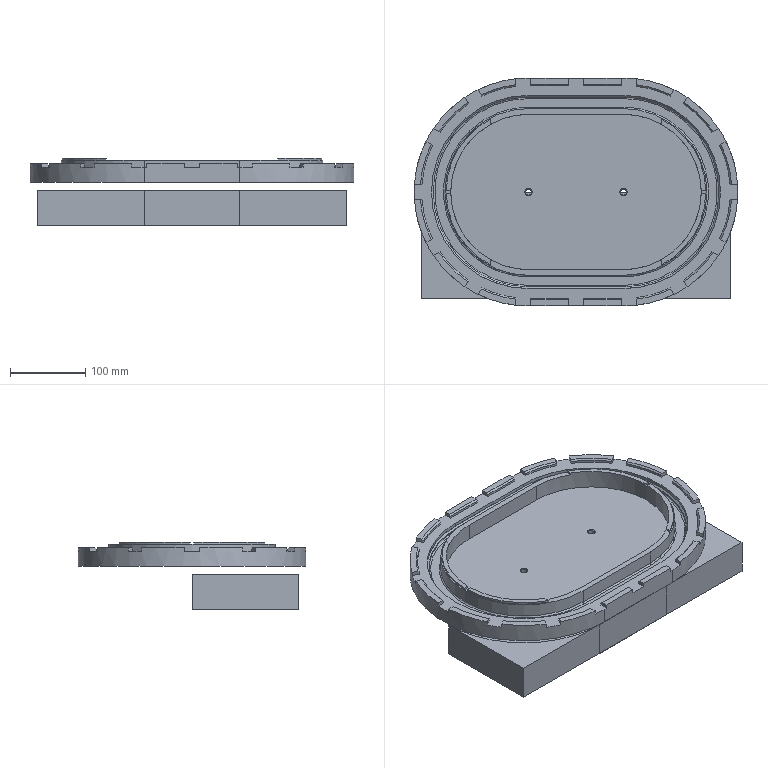NC program | NX | posted with a generic post | part box 429 x 302 x 89.371 mm
Lines 33357 to 34094 of 53366:
(ADAPTIVE_MILLING_COPY , TOOL : D8平刀)
N66710 M6
N66712 G53
N66714 G17 G0 G90 X-179.161 Y14.729 S6500 M3
N66716 G43 Z20. H2
N66718 Z3.
N66720 G94 G3 X-179.161 Y14.729 Z2.673 I-1.578 J-2.534 F3000.
N66722 X-179.161 Y14.729 Z2.345 I-1.578 J-2.534
N66724 X-179.161 Y14.729 Z2.018 I-1.578 J-2.534
N66726 X-179.161 Y14.729 Z1.691 I-1.578 J-2.534
N66728 X-179.161 Y14.729 Z1.363 I-1.578 J-2.534
N66730 X-179.161 Y14.729 Z1.036 I-1.578 J-2.534
N66732 X-179.161 Y14.729 Z0.708 I-1.578 J-2.534
N66734 X-179.161 Y14.729 Z0.381 I-1.578 J-2.534
N66736 X-179.161 Y14.729 Z0.054 I-1.578 J-2.534
N66738 X-179.161 Y14.729 Z-0.274 I-1.578 J-2.534
N66740 X-179.161 Y14.729 Z-0.601 I-1.578 J-2.534
N66742 X-179.161 Y14.729 Z-0.928 I-1.578 J-2.534
N66744 X-179.161 Y14.729 Z-1.256 I-1.578 J-2.534
N66746 X-179.161 Y14.729 Z-1.583 I-1.578 J-2.534
N66748 X-179.161 Y14.729 Z-1.911 I-1.578 J-2.534
N66750 X-179.161 Y14.729 Z-2.238 I-1.578 J-2.534
N66752 X-179.161 Y14.729 Z-2.565 I-1.578 J-2.534
N66754 X-179.161 Y14.729 Z-2.893 I-1.578 J-2.534
N66756 X-179.161 Y14.729 Z-3.22 I-1.578 J-2.534
N66758 X-179.161 Y14.729 Z-3.547 I-1.578 J-2.534
N66760 X-179.161 Y14.729 Z-3.875 I-1.578 J-2.534
N66762 X-179.161 Y14.729 Z-4.202 I-1.578 J-2.534
N66764 X-179.161 Y14.729 Z-4.53 I-1.578 J-2.534
N66766 X-179.161 Y14.729 Z-4.857 I-1.578 J-2.534
N66768 X-179.161 Y14.729 Z-5.184 I-1.578 J-2.534
N66770 X-179.161 Y14.729 Z-5.512 I-1.578 J-2.534
N66772 X-179.161 Y14.729 Z-5.839 I-1.578 J-2.534
N66774 X-179.161 Y14.729 Z-6.166 I-1.578 J-2.534
N66776 X-179.161 Y14.729 Z-6.494 I-1.578 J-2.534
N66778 X-179.161 Y14.729 Z-6.821 I-1.578 J-2.534
N66780 X-179.161 Y14.729 Z-7.148 I-1.578 J-2.534
N66782 X-179.161 Y14.729 Z-7.476 I-1.578 J-2.534
N66784 X-179.161 Y14.729 Z-7.803 I-1.578 J-2.534
N66786 X-179.161 Y14.729 Z-8.131 I-1.578 J-2.534
N66788 X-179.161 Y14.729 Z-8.458 I-1.578 J-2.534
N66790 X-179.161 Y14.729 Z-8.785 I-1.578 J-2.534
N66792 X-179.161 Y14.729 Z-9.113 I-1.578 J-2.534
N66794 X-179.161 Y14.729 Z-9.44 I-1.578 J-2.534
N66796 X-179.161 Y14.729 Z-9.767 I-1.578 J-2.534
N66798 X-179.161 Y14.729 Z-10.095 I-1.578 J-2.534
N66800 X-179.161 Y14.729 Z-10.422 I-1.578 J-2.534
N66802 X-179.161 Y14.729 Z-10.75 I-1.578 J-2.534
N66804 X-179.161 Y14.729 Z-11.077 I-1.578 J-2.534
N66806 X-179.161 Y14.729 Z-11.404 I-1.578 J-2.534
N66808 X-179.161 Y14.729 Z-11.732 I-1.578 J-2.534
N66810 X-179.161 Y14.729 Z-12.059 I-1.578 J-2.534
N66812 X-179.161 Y14.729 Z-12.386 I-1.578 J-2.534
N66814 X-179.161 Y14.729 Z-12.714 I-1.578 J-2.534
N66816 X-179.161 Y14.729 Z-13.041 I-1.578 J-2.534
N66818 X-179.161 Y14.729 Z-13.369 I-1.578 J-2.534
N66820 X-179.161 Y14.729 Z-13.696 I-1.578 J-2.534
N66822 X-179.161 Y14.729 Z-14.023 I-1.578 J-2.534
N66824 X-179.161 Y14.729 Z-14.351 I-1.578 J-2.534
N66826 X-179.161 Y14.729 Z-14.678 I-1.578 J-2.534
N66828 X-179.161 Y14.729 Z-15.005 I-1.578 J-2.534
N66830 X-179.161 Y14.729 Z-15.333 I-1.578 J-2.534
N66832 X-179.161 Y14.729 Z-15.66 I-1.578 J-2.534
N66834 X-179.161 Y14.729 Z-15.988 I-1.578 J-2.534
N66836 X-179.161 Y14.729 Z-16.315 I-1.578 J-2.534
N66838 X-179.161 Y14.729 Z-16.642 I-1.578 J-2.534
N66840 X-179.161 Y14.729 Z-16.97 I-1.578 J-2.534
N66842 X-179.161 Y14.729 Z-17.297 I-1.578 J-2.534
N66844 X-179.161 Y14.729 Z-17.624 I-1.578 J-2.534
N66846 X-179.161 Y14.729 Z-17.952 I-1.578 J-2.534
N66848 X-179.161 Y14.729 Z-18.279 I-1.578 J-2.534
N66850 X-179.161 Y14.729 Z-18.606 I-1.578 J-2.534
N66852 X-179.161 Y14.729 Z-18.934 I-1.578 J-2.534
N66854 X-179.161 Y14.729 Z-19.261 I-1.578 J-2.534
N66856 X-179.161 Y14.729 Z-19.589 I-1.578 J-2.534
N66858 X-179.161 Y14.729 Z-19.916 I-1.578 J-2.534
N66860 X-179.161 Y14.729 Z-20.243 I-1.578 J-2.534
N66862 X-179.161 Y14.729 Z-20.571 I-1.578 J-2.534
N66864 X-179.161 Y14.729 Z-20.898 I-1.578 J-2.534
N66866 X-179.161 Y14.729 Z-21.225 I-1.578 J-2.534
N66868 X-177.814 Y11.601 Z-21.49 R-2.985
N66870 G1 X-177.806 Y12.195 Z-21.5
N66872 G3 X-177.807 Y12.153 R-2.933
N66874 X-177.61 Y12.826 R7.702
N66876 X-178.889 Y15.251 R2.705
N66878 X-183.338 Y14.757 R3.52
N66880 X-183.525 Y14.374 R1.64
N66882 X-183.843 Y11.158 R31.306
N66884 X-181.807 Y8.755 R2.924
N66886 X-177.994 Y9.81 R3.46
N66888 G1 X-177.873 Y10.128
N66890 G2 X-177.489 Y13.792 R46.952
N66892 G3 X-178.725 Y15.899 R2.689
N66894 X-183.073 Y15.946 R3.963
N66896 X-183.386 Y15.443 R1.051
N66898 G1 X-183.531 Y14.327
N66900 X-183.355 Y15.666
N66902 G2 X-182.396 Y16.599 R1.915
N66904 X-177.481 Y15.141 R3.783
N66906 X-177.376 Y14.689 R1.346
N66908 G1 X-177.502 Y13.684
N66910 G3 X-177.335 Y15.196 R17.189
N66912 X-178.575 Y17.058 R2.674
N66914 X-182.918 Y17.15 R3.941
N66916 X-183.228 Y16.65 R1.054
N66918 G1 X-183.374 Y15.534
N66920 X-183.198 Y16.873
N66922 G2 X-182.094 Y17.869 R1.949
N66924 X-177.329 Y16.341 R3.874
N66926 X-177.225 Y15.89 R1.353
N66928 G1 X-177.338 Y14.997
N66930 G3 X-177.186 Y16.401 R11.683
N66932 X-178.441 Y18.238 R2.697
N66934 X-182.659 Y18.421 R3.999
N66936 X-183.071 Y17.848 R0.961
N66938 G1 X-183.217 Y16.732
N66940 X-183.041 Y18.071
N66942 G2 X-182.099 Y18.985 R1.793
N66944 X-177.309 Y17.724 R3.934
N66946 X-177.091 Y16.958 R1.03
N66948 G1 X-177.189 Y16.177
N66950 X-177.023 Y17.356
N66952 G3 X-177.833 Y19.047 R2.299
N66954 X-182.529 Y19.595 R3.989
N66956 X-182.872 Y19.099 R1.038
N66958 G1 X-183.071 Y17.849
N66960 X-182.832 Y19.321
N66962 G2 X-181.691 Y20.279 R1.993
N66964 X-177.101 Y18.819 R3.94
N66966 X-176.89 Y18.131 R1.096
N66968 G1 X-177.023 Y17.355
N66970 G3 X-176.828 Y18.641 R10.399
N66972 X-177.863 Y20.399 R2.573
N66974 X-182.267 Y20.835 R4.01
N66976 X-182.66 Y20.302 R0.982
N66978 G1 X-182.855 Y19.195
N66980 X-182.621 Y20.524
N66982 G2 X-181.478 Y21.469 R1.945
N66984 X-176.799 Y19.79 R3.928
N66986 X-176.692 Y19.284 R1.157
N66988 G1 X-176.844 Y18.397
N66990 G3 X-176.629 Y19.781 R14.102
N66992 X-177.661 Y21.56 R2.598
N66994 X-182.049 Y22.029 R4.
N66996 X-182.451 Y21.492 R0.978
N66998 G1 X-182.646 Y20.384
N67000 X-182.411 Y21.714
N67002 G2 X-181.452 Y22.576 R1.769
N67004 X-176.602 Y20.95 R3.915
N67006 X-176.493 Y20.44 R1.144
N67008 G1 X-176.645 Y19.553
N67010 G3 X-176.429 Y20.932 R20.774
N67012 X-177.551 Y22.801 R2.644
N67014 X-181.826 Y23.219 R3.992
N67016 X-182.243 Y22.675 R0.971
N67018 G1 X-182.438 Y21.567
N67020 X-182.203 Y22.897
N67022 G2 X-181.059 Y23.832 R1.915
N67024 X-176.44 Y22.19 R3.95
N67026 X-176.291 Y21.616 R1.064
N67028 G1 X-176.443 Y20.729
N67030 G3 X-176.23 Y22.123 R11.062
N67032 X-177.388 Y24.002 R2.681
N67034 X-181.597 Y24.408 R4.008
N67036 X-182.088 Y23.556 R1.11
N67038 G1 X-182.224 Y22.78
N67040 X-181.965 Y24.112
N67042 G2 X-180.743 Y25.037 R1.983
N67044 X-176.312 Y23.482 R3.982
N67046 X-176.075 Y22.706 R1.187
N67048 G1 X-176.246 Y21.876
N67050 G3 X-175.993 Y23.214 R12.249
N67052 X-177.023 Y25.05 R2.621
N67054 X-181.304 Y25.624 R4.033
N67056 X-181.747 Y25.099 R0.97
N67058 G1 X-181.99 Y24.001
N67060 X-181.697 Y25.318
N67062 G2 X-180.473 Y26.221 R1.967
N67064 X-175.967 Y24.436 R3.947
N67066 X-175.83 Y23.826 R1.046
N67068 G1 X-176.022 Y22.947
N67070 G3 X-175.747 Y24.343 R9.94
N67072 X-176.794 Y26.216 R2.64
N67074 X-181.056 Y26.793 R4.003
N67076 X-181.486 Y26.273 R0.976
N67078 G1 X-181.73 Y25.175
N67080 X-181.436 Y26.493
N67082 G2 X-180.228 Y27.386 R1.947
N67084 X-175.694 Y25.537 R3.939
N67086 X-175.579 Y24.972 R1.066
N67088 G1 X-175.772 Y24.093
N67090 G3 X-175.496 Y25.484 R9.749
N67092 X-176.607 Y27.425 R2.702
N67094 X-180.739 Y27.994 R4.011
N67096 X-181.226 Y27.443 R0.948
N67098 G1 X-181.47 Y26.345
N67100 X-181.177 Y27.663
N67102 G2 X-180.128 Y28.498 R1.807
N67104 X-175.408 Y26.62 R3.927
N67106 X-175.328 Y26.121 R1.186
N67108 G1 X-175.52 Y25.242
N67110 G3 X-175.243 Y26.649 R10.106
N67112 X-176.368 Y28.594 R2.723
N67114 X-180.507 Y29.145 R4.001
N67116 X-180.967 Y28.611 R0.961
N67118 G1 X-181.211 Y27.512
N67120 X-180.923 Y28.808
N67122 G2 X-179.932 Y29.637 R1.699
N67124 X-175.174 Y27.813 R3.93
N67126 X-175.093 Y27.193 R0.978
N67128 G1 X-175.262 Y26.424
N67130 X-174.991 Y27.576
N67132 G3 X-175.669 Y29.337 R2.307
N67134 X-180.19 Y30.338 R4.018
N67136 X-180.647 Y29.836 R0.974
N67138 G1 X-180.923 Y28.808
N67140 X-180.587 Y30.053
N67142 G2 X-179.342 Y30.901 R1.954
N67144 X-174.955 Y29.053 R3.964
N67146 X-174.793 Y28.318 R1.121
N67148 G1 X-174.996 Y27.557
N67150 G3 X-174.686 Y28.842 R8.026
N67152 X-175.648 Y30.747 R2.648
N67154 X-179.863 Y31.513 R4.006
N67156 X-180.332 Y31.006 R0.968
N67158 G1 X-180.624 Y29.92
N67160 X-180.273 Y31.223
N67162 G2 X-178.977 Y32.073 R1.983
N67164 X-174.554 Y29.953 R3.917
N67166 X-174.494 Y29.442 R1.161
N67168 G1 X-174.726 Y28.572
N67170 G3 X-174.387 Y29.966 R9.375
N67172 X-175.323 Y31.866 R2.649
N67174 X-179.558 Y32.671 R4.006
N67176 X-180.02 Y32.166 R0.971
N67178 G1 X-180.312 Y31.08
N67180 X-179.961 Y32.383
N67182 G2 X-178.764 Y33.205 R1.874
N67184 X-174.272 Y31.141 R3.93
N67186 X-174.19 Y30.581 R1.078
N67188 G1 X-174.422 Y29.712
N67190 G3 X-174.082 Y31.103 R9.82
N67192 X-175.006 Y33. R2.636
N67194 X-179.206 Y33.845 R4.006
N67196 X-179.71 Y33.321 R0.951
N67198 G1 X-180.002 Y32.235
N67200 X-179.651 Y33.538
N67202 G2 X-178.633 Y34.303 R1.758
N67204 X-173.944 Y32.236 R3.928
N67206 X-173.884 Y31.728 R1.17
N67208 G1 X-174.116 Y30.859
N67210 G3 X-173.777 Y32.252 R9.469
N67212 X-174.737 Y34.179 R2.7
N67214 X-178.902 Y34.999 R4.002
N67216 X-179.36 Y34.522 R0.982
N67218 G1 X-179.693 Y33.384
N67220 X-179.291 Y34.737
N67222 G2 X-177.962 Y35.548 R2.008
N67224 X-173.656 Y33.411 R3.93
N67226 X-173.573 Y32.791 R1.031
N67228 G1 X-173.808 Y32.015
N67230 G3 X-173.434 Y33.335 R12.752
N67232 X-174.361 Y35.272 R2.709
N67234 X-178.539 Y36.158 R4.005
N67236 X-178.993 Y35.679 R0.98
N67238 G1 X-179.333 Y34.607
N67240 X-178.925 Y35.894
N67242 G2 X-177.639 Y36.688 R1.942
N67244 X-173.274 Y34.437 R3.932
N67246 X-173.227 Y33.887 R1.084
N67248 G1 X-173.498 Y33.029
N67250 G3 X-173.097 Y34.393 R9.732
N67252 X-173.978 Y36.364 R2.665
N67254 X-178.161 Y37.314 R4.006
N67256 X-178.627 Y36.836 R0.979
N67258 G1 X-178.932 Y35.871
N67260 X-178.558 Y37.051
N67262 G2 X-177.388 Y37.805 R1.844
N67264 X-172.951 Y35.614 R3.933
N67266 X-172.874 Y35.005 R1.058
N67268 G1 X-173.145 Y34.147
N67270 G3 X-172.744 Y35.51 R9.457
N67272 X-173.636 Y37.503 R2.69
N67274 X-177.814 Y38.447 R3.986
N67276 X-178.268 Y37.968 R0.979
N67278 G1 X-178.608 Y36.896
N67280 X-178.2 Y38.183
N67282 G2 X-177.041 Y38.939 R1.818
N67284 X-172.563 Y36.657 R3.941
N67286 X-172.521 Y36.125 R1.116
N67288 G1 X-172.792 Y35.266
N67290 G3 X-172.391 Y36.633 R9.251
N67292 X-173.245 Y38.596 R2.664
N67294 X-177.357 Y39.623 R4.003
N67296 X-177.935 Y39.019 R0.927
N67298 G1 X-178.207 Y38.161
N67300 X-177.811 Y39.362
N67302 G2 X-176.5 Y40.113 R1.968
N67304 X-172.243 Y37.86 R3.943
N67306 X-172.179 Y37.206 R0.993
N67308 G1 X-172.45 Y36.347
N67310 X-172.058 Y37.536
N67312 G3 X-172.523 Y39.291 R2.258
N67314 X-176.969 Y40.77 R4.017
N67316 X-177.464 Y40.311 R0.976
N67318 G1 X-177.85 Y39.255
N67320 X-177.385 Y40.522
N67322 G2 X-176.076 Y41.25 R1.916
N67324 X-171.876 Y38.989 R3.949
N67326 X-171.79 Y38.27 R1.108
N67328 G1 X-172.061 Y37.53
N67330 G3 X-171.637 Y38.776 R8.055
N67332 X-172.487 Y40.83 R2.7
N67334 X-176.501 Y41.917 R3.99
N67336 X-177.051 Y41.439 R0.95
N67338 G1 X-177.438 Y40.382
N67340 X-176.973 Y41.65
N67342 G2 X-175.702 Y42.366 R1.893
N67344 X-171.401 Y39.863 R3.904
N67346 X-171.39 Y39.361 R1.195
N67348 G1 X-171.7 Y38.516
N67350 G3 X-171.234 Y39.873 R9.437
N67352 X-172.071 Y41.926 R2.721
N67354 X-176.171 Y43.013 R3.979
N67356 X-176.641 Y42.558 R0.983
N67358 G1 X-177.028 Y41.501
N67360 X-176.564 Y42.769
N67362 G2 X-175.429 Y43.456 R1.763
N67364 X-171.017 Y41.029 R3.912
N67366 X-170.986 Y40.465 R1.077
N67368 G1 X-171.295 Y39.62
N67370 G3 X-170.834 Y40.954 R11.233
N67372 X-171.651 Y43.02 R2.695
N67374 X-175.757 Y44.134 R3.976
N67376 X-176.232 Y43.675 R0.979
N67378 G1 X-176.58 Y42.724
N67380 X-176.155 Y43.886
N67382 G2 X-174.958 Y44.587 R1.807
N67384 X-170.599 Y42.106 R3.929
N67386 X-170.581 Y41.571 R1.115
N67388 G1 X-170.89 Y40.726
N67390 G3 X-170.426 Y42.083 R9.693
N67392 X-171.14 Y44.015 R2.614
N67394 X-175.269 Y45.275 R3.978
N67396 X-175.766 Y44.84 R0.981
N67398 G1 X-176.178 Y43.824
N67400 X-175.679 Y45.047
N67402 G2 X-174.314 Y45.737 R1.95
N67404 X-170.244 Y43.356 R3.958
N67406 X-170.176 Y42.605 R1.118
N67408 G1 X-170.502 Y41.786
N67410 X-170.045 Y42.917
N67412 G3 X-170.435 Y44.739 R2.278
N67414 X-174.747 Y46.413 R3.997
N67416 X-175.296 Y45.967 R0.96
N67418 G1 X-175.685 Y45.033
N67420 X-175.208 Y46.175
N67422 G2 X-173.921 Y46.833 R1.886
N67424 X-169.737 Y44.22 R3.909
N67426 X-169.734 Y43.661 R1.083
N67428 G1 X-170.081 Y42.831
N67430 G3 X-169.554 Y44.165 R9.887
N67432 X-170.305 Y46.25 R2.709
N67434 X-174.321 Y47.51 R3.984
N67436 X-174.835 Y47.074 R0.976
N67438 G1 X-175.268 Y46.035
N67440 X-174.747 Y47.281
N67442 G2 X-173.47 Y47.933 R1.862
N67444 X-169.279 Y45.274 R3.906
N67446 X-169.285 Y44.735 R1.107
N67448 G1 X-169.632 Y43.905
N67450 G3 X-169.108 Y45.232 R9.499
N67452 X-169.769 Y47.247 R2.645
N67454 X-173.889 Y48.603 R3.964
N67456 X-174.378 Y48.17 R0.985
N67458 G1 X-174.811 Y47.131
N67460 X-174.291 Y48.377
N67462 G2 X-173.119 Y49.014 R1.778
N67464 X-168.832 Y46.384 R3.899
N67466 X-168.829 Y45.825 R1.083
N67468 G1 X-169.176 Y44.995
N67470 G3 X-168.649 Y46.329 R9.634
N67472 X-169.402 Y48.448 R2.735
N67474 X-173.395 Y49.71 R3.969
N67476 X-174.046 Y48.965 R1.17
N67478 G1 X-174.306 Y48.342
N67480 X-173.79 Y49.511
N67482 G2 X-172.452 Y50.138 R1.947
N67484 X-168.365 Y47.439 R3.899
N67486 X-168.373 Y46.914 R1.136
N67488 G1 X-168.72 Y46.084
N67490 X-168.229 Y47.219
N67492 G3 X-168.552 Y49.006 R2.279
N67494 X-172.814 Y50.835 R4.008
N67496 X-173.364 Y50.419 R0.968
N67498 G1 X-173.842 Y49.4
N67500 X-173.267 Y50.622
N67502 G2 X-171.876 Y51.232 R1.963
N67504 X-167.887 Y48.492 R3.89
N67506 X-167.901 Y47.914 R1.065
N67508 G1 X-168.237 Y47.202
N67510 G3 X-167.702 Y48.41 R8.137
N67512 X-168.307 Y50.435 R2.646
N67514 X-172.289 Y51.927 R3.999
N67516 X-172.853 Y51.507 R0.962
N67518 G1 X-173.331 Y50.489
N67520 X-172.756 Y51.71
N67522 G2 X-171.404 Y52.312 R1.928
N67524 X-167.376 Y49.478 R3.889
N67526 X-167.408 Y48.957 R1.143
N67528 G1 X-167.792 Y48.143
N67530 G3 X-167.212 Y49.431 R10.597
N67532 X-167.822 Y51.52 R2.659
N67534 X-171.784 Y53.004 R3.987
N67536 X-172.346 Y52.585 R0.963
N67538 G1 X-172.825 Y51.567
N67540 X-172.25 Y52.788
N67542 G2 X-171.036 Y53.372 R1.821
N67544 X-166.884 Y50.563 R3.897
N67546 X-166.91 Y50.009 R1.083
N67548 G1 X-167.295 Y49.195
N67550 G3 X-166.71 Y50.505 R9.831
N67552 X-167.309 Y52.571 R2.682
N67554 X-171.33 Y54.068 R3.963
N67556 X-171.844 Y53.654 R0.979
N67558 G1 X-172.322 Y52.636
N67560 X-171.699 Y53.93
N67562 G2 X-170.064 Y54.475 R2.216
N67564 X-166.378 Y51.607 R3.911
N67566 X-166.408 Y51.071 R1.111
N67568 G1 X-166.793 Y50.258
N67570 G3 X-166.21 Y51.558 R9.537
N67572 X-166.828 Y53.67 R2.695
N67574 X-170.711 Y55.174 R4.003
N67576 X-171.259 Y54.785 R0.978
N67578 G1 X-171.758 Y53.834
N67580 X-171.154 Y54.984
N67582 G2 X-169.965 Y55.523 R1.831
N67584 X-165.85 Y52.562 R3.881
N67586 X-165.908 Y52.076 R1.24
N67588 G1 X-166.289 Y51.324
N67590 X-165.751 Y52.375
N67592 G3 X-166.013 Y54.281 R2.322
N67594 X-170.207 Y56.226 R3.947
N67596 X-170.698 Y55.853 R1.022
N67598 G1 X-171.221 Y54.857
N67600 X-170.593 Y56.052
N67602 G2 X-169.355 Y56.586 R1.809
N67604 X-165.328 Y53.633 R3.883
N67606 X-165.378 Y53.08 R1.087
N67608 G1 X-165.798 Y52.284
N67610 X-165.176 Y53.482
N67612 G3 X-165.568 Y55.487 R2.541
N67614 X-169.611 Y57.297 R3.969
N67616 X-170.145 Y56.908 R0.981
N67618 G1 X-170.668 Y55.912
N67620 X-170.04 Y57.107
N67622 G2 X-168.854 Y57.636 R1.782
N67624 X-164.778 Y54.615 R3.87
N67626 X-164.833 Y54.11 R1.179
N67628 G1 X-165.254 Y53.314
N67630 G3 X-164.613 Y54.595 R9.431
N67632 X-165.159 Y56.739 R2.719
N67634 X-169.088 Y58.342 R3.936
N67636 X-169.59 Y57.964 R1.009
N67638 G1 X-170.113 Y56.968
N67640 X-169.485 Y58.163
N67642 G2 X-168.197 Y58.699 R1.847
N67644 X-164.229 Y55.661 R3.891
N67646 X-164.284 Y55.15 R1.16
N67648 G1 X-164.705 Y54.354
N67650 G3 X-164.065 Y55.625 R10.234
N67652 X-164.53 Y57.669 R2.661
N67654 X-168.486 Y59.405 R3.952
N67656 X-168.988 Y59.056 R1.027
N67658 G1 X-169.544 Y58.051
N67660 X-168.874 Y59.25
N67662 G2 X-167.363 Y59.754 R2.037
N67664 X-163.682 Y56.717 R3.903
N67666 X-163.759 Y56.143 R1.019
N67668 G1 X-164.127 Y55.447
N67670 G3 X-163.515 Y56.616 R13.972
N67672 X-163.989 Y58.735 R2.644
N67674 X-167.851 Y60.463 R3.956
N67676 X-168.376 Y60.106 R1.001
N67678 G1 X-168.943 Y59.134
N67680 X-168.262 Y60.3
N67682 G2 X-166.79 Y60.789 R1.964
N67684 X-163.146 Y57.876 R3.919
N67686 X-163.182 Y57.127 R1.139
N67688 G1 X-163.58 Y56.447
N67690 G3 X-162.945 Y57.583 R9.285
N67692 X-163.337 Y59.651 R2.605
N67694 X-167.273 Y61.49 R3.928
N67696 X-167.771 Y61.143 R1.033
N67698 G1 X-168.338 Y60.171
N67700 X-167.657 Y61.337
N67702 G2 X-166.431 Y61.812 R1.808
N67704 X-162.53 Y58.715 R3.873
N67706 X-162.593 Y58.131 R1.061
N67708 G1 X-163.048 Y57.354
N67710 G3 X-162.356 Y58.589 R9.693
N67712 X-162.808 Y60.763 R2.666
N67714 X-166.691 Y62.515 R3.898
N67716 X-167.171 Y62.174 R1.055
N67718 G1 X-167.737 Y61.202
N67720 X-167.056 Y62.367
N67722 G2 X-165.796 Y62.839 R1.838
N67724 X-161.929 Y59.692 R3.883
N67726 X-162.001 Y59.139 R1.085
N67728 G1 X-162.457 Y58.363
N67730 G3 X-161.762 Y59.603 R9.487
N67732 X-162.211 Y61.777 R2.689
N67734 X-165.993 Y63.561 R3.941
N67736 X-166.581 Y63.185 R0.958
N67738 G1 X-167.148 Y62.213
N67740 X-166.438 Y63.408
N67742 G2 X-164.978 Y63.866 R1.98
N67744 X-161.327 Y60.644 R3.881
N67746 X-161.406 Y60.154 R1.216
N67748 G1 X-161.862 Y59.378
N67750 G3 X-161.163 Y60.63 R9.871
N67752 X-161.616 Y62.8 R2.704
N67754 X-165.364 Y64.589 R3.948
N67756 X-165.889 Y64.26 R1.018
N67758 G1 X-166.498 Y63.314
N67760 X-165.767 Y64.449
N67762 G2 X-164.24 Y64.872 R2.025
N67764 X-160.734 Y61.676 R3.876
N67766 X-160.822 Y61.093 R1.052
N67768 G1 X-161.289 Y60.353
N67770 X-160.639 Y61.376
N67772 G3 X-160.711 Y63.262 R2.285
N67774 X-164.661 Y65.611 R3.952
N67776 X-165.237 Y65.272 R0.979
N67778 G1 X-165.847 Y64.326
N67780 X-165.115 Y65.461
N67782 G2 X-163.877 Y65.883 R1.796
N67784 X-160.098 Y62.544 R3.853
N67786 X-160.199 Y62.055 R1.205
N67788 G1 X-160.688 Y61.3
N67790 G3 X-159.937 Y62.518 R9.015
N67792 X-160.303 Y64.687 R2.66
N67794 X-164.068 Y66.602 R3.899
N67796 X-164.593 Y66.273 R1.018
N67798 G1 X-165.202 Y65.327
N67800 X-164.47 Y66.462
N67802 G2 X-163.224 Y66.884 R1.816
N67804 X-159.465 Y63.49 R3.856
N67806 X-159.567 Y63.03 R1.312
N67808 G1 X-160.056 Y62.275
N67810 G3 X-159.311 Y63.475 R10.277
N67812 X-159.617 Y65.597 R2.626
N67814 X-163.359 Y67.611 R3.922
N67816 X-163.949 Y67.272 R0.973
N67818 G1 X-164.559 Y66.326
N67820 X-163.827 Y67.46
N67822 G2 X-162.375 Y67.876 R1.946
N67824 X-158.831 Y64.542 R3.881
N67826 X-158.932 Y64.012 R1.104
N67828 G1 X-159.421 Y63.256
N67830 G3 X-158.67 Y64.471 R10.085
N67832 X-159.044 Y66.7 R2.7
N67834 X-162.682 Y68.614 R3.94
N67836 X-163.249 Y68.301 R0.99
N67838 G1 X-163.92 Y67.317
N67840 X-163.118 Y68.484
N67842 G2 X-161.61 Y68.853 R2.
N67844 X-158.229 Y65.795 R3.928
N67846 X-158.4 Y64.833 R1.096
N67848 G1 X-158.767 Y64.266
N67850 X-158.112 Y65.237
N67852 G3 X-158.12 Y67.135 R2.289
N67854 X-161.963 Y69.602 R3.939
N67856 X-162.548 Y69.289 R0.982
N67858 G1 X-163.199 Y68.371
N67860 X-162.418 Y69.472
N67862 G2 X-160.997 Y69.838 R1.917
N67864 X-157.556 Y66.649 R3.892
N67866 X-157.66 Y65.872 R1.162
N67868 G1 X-158.117 Y65.23
N67870 G3 X-157.378 Y66.318 R8.566
N67872 X-157.644 Y68.512 R2.649
N67874 X-161.333 Y70.569 R3.884
N67876 X-161.854 Y70.268 R1.04
N67878 G1 X-162.504 Y69.351
N67880 X-161.723 Y70.451
N67882 G2 X-160.246 Y70.802 R1.942
N67884 X-156.877 Y67.527 R3.889
N67886 X-156.984 Y66.82 R1.125
N67888 G1 X-157.506 Y66.087
N67890 G3 X-156.707 Y67.251 R11.446
N67892 X-156.919 Y69.381 R2.632
N67894 X-160.545 Y71.551 R3.933
N67896 X-161.166 Y71.238 R0.965
N67898 G1 X-161.817 Y70.32
N67900 X-161.035 Y71.421
N67902 G2 X-159.722 Y71.782 R1.821
N67904 X-156.185 Y68.3 R3.859
N67906 X-156.31 Y67.766 R1.09
N67908 G1 X-156.832 Y67.033
N67910 G3 X-156.035 Y68.19 R15.218
N67912 X-156.294 Y70.444 R2.685
N67914 X-159.916 Y72.514 R3.891
N67916 X-160.574 Y72.073 R0.975
N67918 G1 X-161.16 Y71.247
N67920 X-160.309 Y72.414
N67922 G2 X-158.85 Y72.731 R1.976
N67924 X-155.503 Y69.231 R3.852
N67926 X-155.626 Y68.726 R1.147
N67928 G1 X-156.149 Y67.993
N67930 G3 X-155.348 Y69.164 R10.165
N67932 X-155.602 Y71.389 R2.686
N67934 X-159.219 Y73.472 R3.856
N67936 X-159.701 Y73.198 R1.082
N67938 G1 X-160.392 Y72.31
N67940 X-159.563 Y73.375
N67942 G2 X-158.101 Y73.677 R1.934
N67944 X-154.82 Y70.161 R3.848
N67946 X-154.961 Y69.6 R1.065
N67948 G1 X-155.437 Y68.991
N67950 G3 X-154.663 Y70.032 R7.555
N67952 X-154.836 Y72.207 R2.644
N67954 X-158.402 Y74.431 R3.92
N67956 X-158.961 Y74.149 R1.01
N67958 G1 X-159.583 Y73.349
N67960 X-158.823 Y74.326
N67962 G2 X-157.353 Y74.615 R1.904
N67964 X-154.117 Y71.177 R3.879
N67966 X-154.255 Y70.505 R1.102
N67968 G1 X-154.809 Y69.795
N67970 G3 X-153.953 Y70.941 R9.388
N67972 X-154.156 Y73.204 R2.696
N67974 X-157.605 Y75.373 R3.928
N67976 X-158.231 Y75.088 R0.969
N67978 G1 X-158.922 Y74.2
N67980 X-158.092 Y75.265
N67982 G2 X-156.597 Y75.543 R1.932
N67984 X-153.397 Y71.96 R3.863
N67986 X-153.541 Y71.418 R1.081
N67988 G1 X-154.095 Y70.709
N67990 G3 X-153.239 Y71.854 R9.69
N67992 X-153.382 Y74.021 R2.658
N67994 X-156.959 Y76.3 R3.879
N67996 X-157.506 Y76.02 R1.023
N67998 G1 X-158.197 Y75.132
N68000 X-157.367 Y76.197
N68002 G2 X-156.07 Y76.499 R1.788
N68004 X-152.677 Y72.844 R3.848
N68006 X-152.823 Y72.336 R1.128
N68008 G1 X-153.377 Y71.627
N68010 G3 X-152.52 Y72.772 R10.162
N68012 X-152.707 Y75.048 R2.72
N68014 X-156.103 Y77.239 R3.932
N68016 X-156.712 Y76.978 R0.982
N68018 G1 X-157.488 Y76.043
N68020 X-156.566 Y77.149
N68022 G2 X-155.076 Y77.387 R1.948
N68024 X-151.955 Y73.756 R3.845
N68026 X-152.293 Y73.014 R1.03
N68028 G1 X-152.64 Y72.571
N68030 X-151.903 Y73.471
N68032 G3 X-151.755 Y75.423 R2.322
N68034 X-155.315 Y78.156 R3.928
N68036 X-155.93 Y77.897 R0.979
N68038 G1 X-156.66 Y77.041
N68040 X-155.784 Y78.068
N68042 G2 X-154.306 Y78.295 R1.915
N68044 X-151.222 Y74.549 R3.827
N68046 X-151.387 Y74.074 R1.194
N68048 G1 X-151.972 Y73.39
N68050 G3 X-151.072 Y74.488 R10.029
N68052 X-151.136 Y76.675 R2.662
N68054 X-154.538 Y79.064 R3.908
N68056 X-155.157 Y78.805 R0.978
N68058 G1 X-155.886 Y77.948
N68060 X-155.011 Y78.976
N68062 G2 X-153.646 Y79.213 R1.847
N68064 X-150.472 Y75.445 R3.823
N68066 X-150.64 Y74.947 R1.135
N68068 G1 X-151.225 Y74.263
N68070 G3 X-150.328 Y75.348 R12.911
N68072 X-150.373 Y77.554 R2.66
N68074 X-153.764 Y79.963 R3.909
N68076 X-154.39 Y79.705 R0.975
N68078 G1 X-155.12 Y78.849
N68080 X-154.244 Y79.876
N68082 G2 X-152.758 Y80.091 R1.91
N68084 X-149.713 Y76.334 R3.851
N68086 X-149.881 Y75.834 R1.131
N68088 G1 X-150.466 Y75.15
N68090 G3 X-149.569 Y76.237 R12.034
N68092 X-149.581 Y78.365 R2.643
N68094 X-152.987 Y80.862 R3.907
N68096 X-153.803 Y80.395 R1.047
N68098 G1 X-154.387 Y79.709
N68100 X-153.435 Y80.791
N68102 G2 X-151.879 Y80.964 R1.973
N68104 X-148.958 Y77.178 R3.844
N68106 X-149.121 Y76.723 R1.265
N68108 G1 X-149.706 Y76.039
N68110 G3 X-148.805 Y77.123 R11.07
N68112 X-148.856 Y79.348 R2.693
N68114 X-152.2 Y81.75 R3.876
N68116 X-152.755 Y81.522 R1.042
N68118 G1 X-153.445 Y80.781
N68120 X-152.601 Y81.686
N68122 G2 X-151.135 Y81.852 R1.916
N68124 X-148.189 Y78.236 R3.862
N68126 X-148.386 Y77.524 R1.126
N68128 G1 X-148.924 Y76.949
N68130 G3 X-148.054 Y77.921 R8.622
N68132 X-148.057 Y80.178 R2.687
N68134 X-151.403 Y82.625 R3.869
N68136 X-151.939 Y82.398 R1.06
N68138 G1 X-152.706 Y81.575
N68140 X-151.785 Y82.562
N68142 G2 X-150.461 Y82.745 R1.816
N68144 X-147.417 Y78.838 R3.816
N68146 X-147.605 Y78.359 R1.161
N68148 G1 X-148.22 Y77.702
N68150 G3 X-147.275 Y78.749 R11.226
N68152 X-147.21 Y80.891 R2.629
N68154 X-150.558 Y83.491 R3.877
N68156 X-151.137 Y83.259 R1.014
N68158 G1 X-151.904 Y82.436
N68160 X-150.983 Y83.423
N68162 G2 X-149.493 Y83.574 R1.895
N68164 X-146.629 Y79.658 R3.825
N68166 X-146.812 Y79.207 R1.251
N68168 G1 X-147.427 Y78.55
N68170 G3 X-146.475 Y79.611 R10.161
N68172 X-146.454 Y81.856 R2.702
N68174 X-149.705 Y84.355 R3.908
N68176 X-150.332 Y84.124 R0.979
N68178 G1 X-151.099 Y83.3